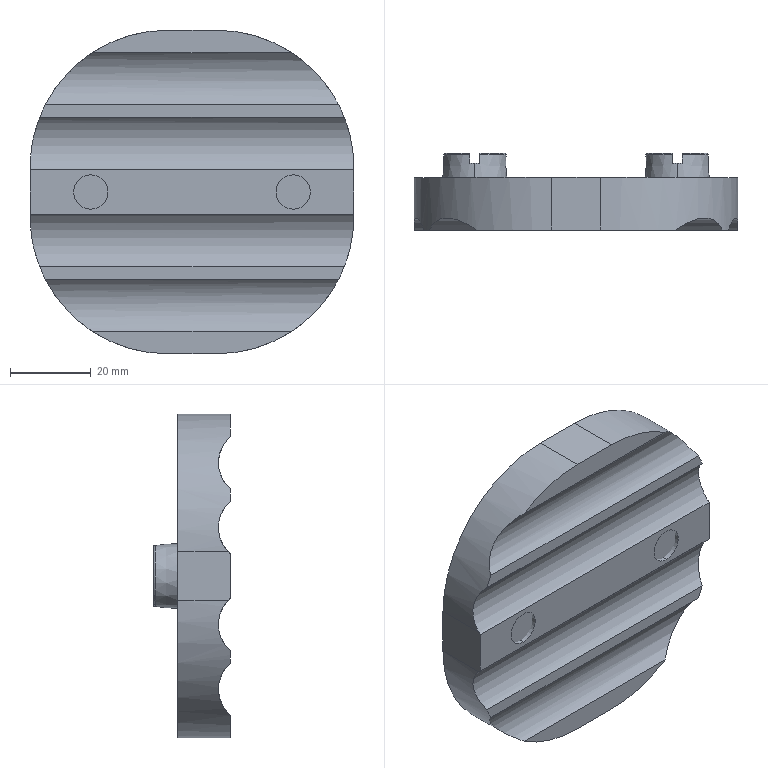Part | SolidWorks | features MirrorStock 1 | 3 solids | 52 faces | box 80 x 19 x 80 mm | volume 65180 mm3 | plane 24 | cylinder 16 | torus 8 | cone 4 | commonest cylinder face diameters 8.5 x4 10 x4 17 x4 68 x4